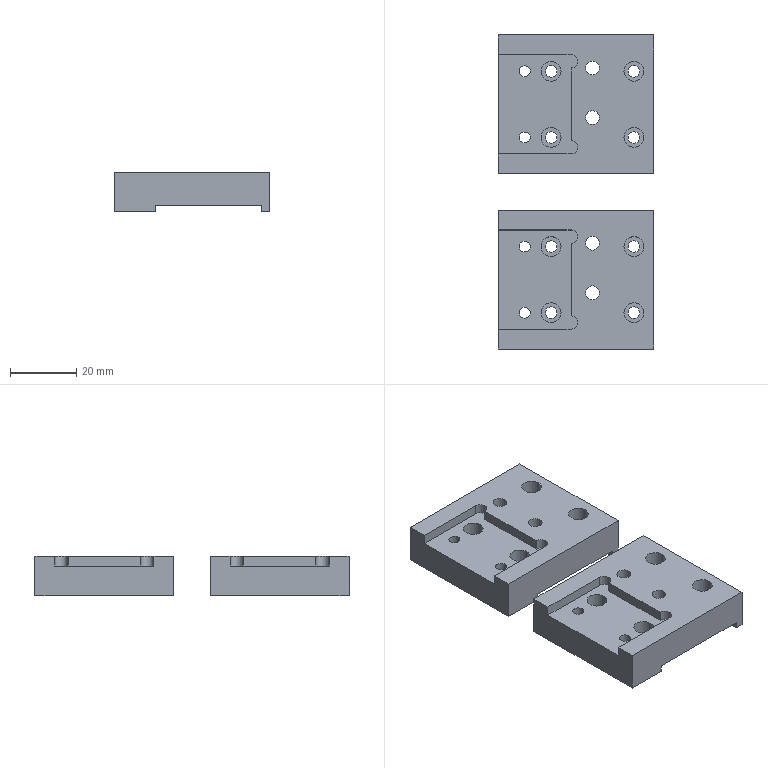NC program | NX | posted with a generic post | part box 47 x 95 x 12 mm
Lines 1783 to 2681 of 2681:
(FLOOR_WALL_COPY , TOOL : D10JING)
N3528 T14 M6
N3530 G54
N3532 G17 G0 G90 X-34.9 Y-30. S9500 M3
N3534 G43 Z30. H14
N3536 Z-1.5
N3538 G94 G1 Z-3. F1500.
N3540 X-35.399 Y-27.634
N3542 G3 X-35.899 Y-28.5 R1.
N3544 G1 Y-7.1
N3546 X-31.199
N3548 Y-28.5
N3550 X-26.5
N3552 Y-7.1
N3554 X-21.8
N3556 Y-28.5
N3558 X-17.1
N3560 Y-7.1
N3562 G3 X-17.966 Y-7.6 R1.
N3564 G1 Z-1.5
N3566 G0 X-18.198 Y-30.
N3568 G1 Z-3.
N3570 X-17.1 Y-29.366
N3572 G3 X-16.6 Y-28.5 R1.
N3574 G1 Y-6.6
N3576 X-36.4
N3578 Y-28.5
N3580 G3 X-35.9 Y-29.366 R1.
N3582 G1 X-34.802 Y-30.
N3584 Z-1.5
N3586 G0 Z0.1
N3588 X18.1
N3590 Z-1.5
N3592 G1 Z-3.
N3594 X17.601 Y-27.634
N3596 G3 X17.101 Y-28.5 R1.
N3598 G1 Y-7.1
N3600 X21.801
N3602 Y-28.5
N3604 X26.5
N3606 Y-7.1
N3608 X31.2
N3610 Y-28.5
N3612 X35.9
N3614 Y-7.1
N3616 G3 X35.034 Y-7.6 R1.
N3618 G1 Z-1.5
N3620 G0 X34.802 Y-30.
N3622 G1 Z-3.
N3624 X35.9 Y-29.366
N3626 G3 X36.4 Y-28.5 R1.
N3628 G1 Y-6.6
N3630 X16.6
N3632 Y-28.5
N3634 G3 X17.1 Y-29.366 R1.
N3636 G1 X18.198 Y-30.
N3638 Z-1.5
N3640 G0 Z30.
(ZLEVEL_PROFILE_COPY_1 , TOOL : D10JING)
N3642 X-0.5 Y-4.296
N3644 Z1.5
N3646 G1 Y-24.049 Z0.465 F1000.
N3648 X-0.828 Y-25.364 Z0.394
N3650 X-1.496 Y-26.545 Z0.323
N3652 X-2.455 Y-27.504 Z0.252
N3654 X-3.636 Y-28.172 Z0.18
N3656 X-4.951 Y-28.5 Z0.109
N3658 X-48.049 Z-2.149
N3660 X-49.364 Y-28.172 Z-2.22
N3662 X-50.545 Y-27.504 Z-2.291
N3664 X-51.504 Y-26.545 Z-2.362
N3666 X-52.172 Y-25.364 Z-2.434
N3668 X-52.5 Y-24.049 Z-2.505
N3670 Y24.049 Z-5.025
N3672 X-52.172 Y25.364 Z-5.096
N3674 X-51.504 Y26.545 Z-5.167
N3676 X-50.545 Y27.504 Z-5.238
N3678 X-49.364 Y28.172 Z-5.31
N3680 X-48.049 Y28.5 Z-5.381
N3682 X-4.951 Z-7.639
N3684 X-3.636 Y28.172 Z-7.71
N3686 X-2.455 Y27.504 Z-7.781
N3688 X-1.496 Y26.545 Z-7.852
N3690 X-0.828 Y25.364 Z-7.924
N3692 X-0.5 Y24.049 Z-7.995
N3694 Y-24.049 Z-10.515
N3696 X-0.828 Y-25.364 Z-10.586
N3698 X-1.496 Y-26.545 Z-10.657
N3700 X-2.455 Y-27.504 Z-10.729
N3702 X-3.636 Y-28.172 Z-10.8
N3704 X-4.951 Y-28.5 Z-10.871
N3706 X-26.5 Z-12.
N3708 X-47.5 F1200.
N3710 G2 X-52.5 Y-23.5 R5.
N3712 G1 Y23.5
N3714 G2 X-47.5 Y28.5 R5.
N3716 G1 X-5.5
N3718 G2 X-0.5 Y23.5 R5.
N3720 G1 Y-23.5
N3722 G2 X-5.5 Y-28.5 R5.
N3724 G1 X-26.5
N3726 Z-10.5
N3728 G0 Z53.
N3730 X52.5 Y-4.296
N3732 Z1.5
N3734 G1 Y-24.049 Z0.465 F1000.
N3736 X52.172 Y-25.364 Z0.394
N3738 X51.504 Y-26.545 Z0.323
N3740 X50.545 Y-27.504 Z0.252
N3742 X49.364 Y-28.172 Z0.18
N3744 X48.049 Y-28.5 Z0.109
N3746 X4.951 Z-2.149
N3748 X3.636 Y-28.172 Z-2.22
N3750 X2.455 Y-27.504 Z-2.291
N3752 X1.496 Y-26.545 Z-2.362
N3754 X0.828 Y-25.364 Z-2.434
N3756 X0.5 Y-24.049 Z-2.505
N3758 Y24.049 Z-5.025
N3760 X0.828 Y25.364 Z-5.096
N3762 X1.496 Y26.545 Z-5.167
N3764 X2.455 Y27.504 Z-5.238
N3766 X3.636 Y28.172 Z-5.31
N3768 X4.951 Y28.5 Z-5.381
N3770 X48.049 Z-7.639
N3772 X49.364 Y28.172 Z-7.71
N3774 X50.545 Y27.504 Z-7.781
N3776 X51.504 Y26.545 Z-7.852
N3778 X52.172 Y25.364 Z-7.924
N3780 X52.5 Y24.049 Z-7.995
N3782 Y-24.049 Z-10.515
N3784 X52.172 Y-25.364 Z-10.586
N3786 X51.504 Y-26.545 Z-10.657
N3788 X50.545 Y-27.504 Z-10.729
N3790 X49.364 Y-28.172 Z-10.8
N3792 X48.049 Y-28.5 Z-10.871
N3794 X26.5 Z-12.
N3796 X5.5 F1200.
N3798 G2 X0.5 Y-23.5 R5.
N3800 G1 Y23.5
N3802 G2 X5.5 Y28.5 R5.
N3804 G1 X47.5
N3806 G2 X52.5 Y23.5 R5.
N3808 G1 Y-23.5
N3810 G2 X47.5 Y-28.5 R5.
N3812 G1 X26.5
N3814 Z-10.5
N3816 G0 Z30.
N3818 M5
(HOLE_MILLING , TOOL : D4)
N3820 T11 M6
N3822 G54
N3824 G17 G0 G90 X-36.5 Y17.5 S9500 M3
N3826 G43 Z30. H11
N3828 Z0.5
N3830 G94 G3 X-36. Y18. R0.5 F1600.
N3832 X-36.5 Y18.5 R0.5
N3834 X-36.5 Y18.5 Z0.1 I0. J-1.
N3836 X-36.5 Y18.5 Z-0.3 I0. J-1.
N3838 X-36.5 Y18.5 Z-0.7 I0. J-1.
N3840 X-36.5 Y18.5 Z-1.1 I0. J-1.
N3842 X-36.5 Y18.5 Z-1.5 I0. J-1.
N3844 X-36.5 Y18.5 Z-1.9 I0. J-1.
N3846 X-36.5 Y18.5 Z-2.3 I0. J-1.
N3848 X-36.5 Y18.5 Z-2.7 I0. J-1.
N3850 X-36.5 Y18.5 Z-3.1 I0. J-1.
N3852 X-36.5 Y18.5 Z-3.5 I0. J-1.
N3854 X-36.5 Y18.5 Z-3.9 I0. J-1.
N3856 X-36.5 Y18.5 Z-4.3 I0. J-1.
N3858 X-36.5 Y18.5 Z-4.7 I0. J-1.
N3860 X-36.5 Y18.5 Z-5.1 I0. J-1.
N3862 X-36.5 Y18.5 Z-5.5 I0. J-1.
N3864 X-36.5 Y18.5 Z-5.9 I0. J-1.
N3866 X-36.5 Y18.5 Z-6.3 I0. J-1.
N3868 X-36.5 Y18.5 Z-6.7 I0. J-1.
N3870 X-36.5 Y18.5 Z-7.1 I0. J-1.
N3872 X-36.5 Y18.5 Z-7.5 I0. J-1.
N3874 X-36.5 Y18.5 Z-7.9 I0. J-1.
N3876 X-37.5 Y17.5 Z-8. R1.
N3878 X-36.5 Y16.5 R1.
N3880 X-37.5 Y17.5 R-1.
N3882 X-37. Y17. R0.5
N3884 X-36.5 Y17.5 R0.5
N3886 G0 Z30.
N3888 Y-7.5
N3890 Z-2.5
N3892 G3 X-36. Y-7. R0.5
N3894 X-36.5 Y-6.5 R0.5
N3896 X-36.5 Y-6.5 Z-2.9 I0. J-1.
N3898 X-36.5 Y-6.5 Z-3.3 I0. J-1.
N3900 X-36.5 Y-6.5 Z-3.7 I0. J-1.
N3902 X-36.5 Y-6.5 Z-4.1 I0. J-1.
N3904 X-36.5 Y-6.5 Z-4.5 I0. J-1.
N3906 X-36.5 Y-6.5 Z-4.9 I0. J-1.
N3908 X-36.5 Y-6.5 Z-5.3 I0. J-1.
N3910 X-36.5 Y-6.5 Z-5.7 I0. J-1.
N3912 X-36.5 Y-6.5 Z-6.1 I0. J-1.
N3914 X-36.5 Y-6.5 Z-6.5 I0. J-1.
N3916 X-36.5 Y-6.5 Z-6.9 I0. J-1.
N3918 X-36.5 Y-6.5 Z-7.3 I0. J-1.
N3920 X-36.5 Y-6.5 Z-7.7 I0. J-1.
N3922 X-35.5 Y-7.5 Z-8. R-1.
N3924 X-36.5 Y-6.5 R1.
N3926 X-35.5 Y-7.5 R-1.
N3928 X-36. Y-7. R0.5
N3930 X-36.5 Y-7.5 R0.5
N3932 G0 Z30.
N3934 X-16.5
N3936 Z-2.5
N3938 G3 X-16. Y-7. R0.5
N3940 X-16.5 Y-6.5 R0.5
N3942 X-16.5 Y-6.5 Z-2.9 I0. J-1.
N3944 X-16.5 Y-6.5 Z-3.3 I0. J-1.
N3946 X-16.5 Y-6.5 Z-3.7 I0. J-1.
N3948 X-16.5 Y-6.5 Z-4.1 I0. J-1.
N3950 X-16.5 Y-6.5 Z-4.5 I0. J-1.
N3952 X-16.5 Y-6.5 Z-4.9 I0. J-1.
N3954 X-16.5 Y-6.5 Z-5.3 I0. J-1.
N3956 X-16.5 Y-6.5 Z-5.7 I0. J-1.
N3958 X-16.5 Y-6.5 Z-6.1 I0. J-1.
N3960 X-16.5 Y-6.5 Z-6.5 I0. J-1.
N3962 X-16.5 Y-6.5 Z-6.9 I0. J-1.
N3964 X-16.5 Y-6.5 Z-7.3 I0. J-1.
N3966 X-16.5 Y-6.5 Z-7.7 I0. J-1.
N3968 X-15.5 Y-7.5 Z-8. R-1.
N3970 X-16.5 Y-6.5 R1.
N3972 X-15.5 Y-7.5 R-1.
N3974 X-16. Y-7. R0.5
N3976 X-16.5 Y-7.5 R0.5
N3978 G0 Z30.
N3980 Y17.5
N3982 Z0.5
N3984 G3 X-16. Y18. R0.5
N3986 X-16.5 Y18.5 R0.5
N3988 X-16.5 Y18.5 Z0.1 I0. J-1.
N3990 X-16.5 Y18.5 Z-0.3 I0. J-1.
N3992 X-16.5 Y18.5 Z-0.7 I0. J-1.
N3994 X-16.5 Y18.5 Z-1.1 I0. J-1.
N3996 X-16.5 Y18.5 Z-1.5 I0. J-1.
N3998 X-16.5 Y18.5 Z-1.9 I0. J-1.
N4000 X-16.5 Y18.5 Z-2.3 I0. J-1.
N4002 X-16.5 Y18.5 Z-2.7 I0. J-1.
N4004 X-16.5 Y18.5 Z-3.1 I0. J-1.
N4006 X-16.5 Y18.5 Z-3.5 I0. J-1.
N4008 X-16.5 Y18.5 Z-3.9 I0. J-1.
N4010 X-16.5 Y18.5 Z-4.3 I0. J-1.
N4012 X-16.5 Y18.5 Z-4.7 I0. J-1.
N4014 X-16.5 Y18.5 Z-5.1 I0. J-1.
N4016 X-16.5 Y18.5 Z-5.5 I0. J-1.
N4018 X-16.5 Y18.5 Z-5.9 I0. J-1.
N4020 X-16.5 Y18.5 Z-6.3 I0. J-1.
N4022 X-16.5 Y18.5 Z-6.7 I0. J-1.
N4024 X-16.5 Y18.5 Z-7.1 I0. J-1.
N4026 X-16.5 Y18.5 Z-7.5 I0. J-1.
N4028 X-16.5 Y18.5 Z-7.9 I0. J-1.
N4030 X-17.5 Y17.5 Z-8. R1.
N4032 X-16.5 Y16.5 R1.
N4034 X-17.5 Y17.5 R-1.
N4036 X-17. Y17. R0.5
N4038 X-16.5 Y17.5 R0.5
N4040 G0 Z30.
N4042 X16.5
N4044 Z0.5
N4046 G3 X17. Y18. R0.5
N4048 X16.5 Y18.5 R0.5
N4050 X16.5 Y18.5 Z0.1 I0. J-1.
N4052 X16.5 Y18.5 Z-0.3 I0. J-1.
N4054 X16.5 Y18.5 Z-0.7 I0. J-1.
N4056 X16.5 Y18.5 Z-1.1 I0. J-1.
N4058 X16.5 Y18.5 Z-1.5 I0. J-1.
N4060 X16.5 Y18.5 Z-1.9 I0. J-1.
N4062 X16.5 Y18.5 Z-2.3 I0. J-1.
N4064 X16.5 Y18.5 Z-2.7 I0. J-1.
N4066 X16.5 Y18.5 Z-3.1 I0. J-1.
N4068 X16.5 Y18.5 Z-3.5 I0. J-1.
N4070 X16.5 Y18.5 Z-3.9 I0. J-1.
N4072 X16.5 Y18.5 Z-4.3 I0. J-1.
N4074 X16.5 Y18.5 Z-4.7 I0. J-1.
N4076 X16.5 Y18.5 Z-5.1 I0. J-1.
N4078 X16.5 Y18.5 Z-5.5 I0. J-1.
N4080 X16.5 Y18.5 Z-5.9 I0. J-1.
N4082 X16.5 Y18.5 Z-6.3 I0. J-1.
N4084 X16.5 Y18.5 Z-6.7 I0. J-1.
N4086 X16.5 Y18.5 Z-7.1 I0. J-1.
N4088 X16.5 Y18.5 Z-7.5 I0. J-1.
N4090 X16.5 Y18.5 Z-7.9 I0. J-1.
N4092 X15.5 Y17.5 Z-8. R1.
N4094 X16.5 Y16.5 R1.
N4096 X15.5 Y17.5 R-1.
N4098 X16. Y17. R0.5
N4100 X16.5 Y17.5 R0.5
N4102 G0 Z30.
N4104 X36.5
N4106 Z0.5
N4108 G3 X37. Y18. R0.5
N4110 X36.5 Y18.5 R0.5
N4112 X36.5 Y18.5 Z0.1 I0. J-1.
N4114 X36.5 Y18.5 Z-0.3 I0. J-1.
N4116 X36.5 Y18.5 Z-0.7 I0. J-1.
N4118 X36.5 Y18.5 Z-1.1 I0. J-1.
N4120 X36.5 Y18.5 Z-1.5 I0. J-1.
N4122 X36.5 Y18.5 Z-1.9 I0. J-1.
N4124 X36.5 Y18.5 Z-2.3 I0. J-1.
N4126 X36.5 Y18.5 Z-2.7 I0. J-1.
N4128 X36.5 Y18.5 Z-3.1 I0. J-1.
N4130 X36.5 Y18.5 Z-3.5 I0. J-1.
N4132 X36.5 Y18.5 Z-3.9 I0. J-1.
N4134 X36.5 Y18.5 Z-4.3 I0. J-1.
N4136 X36.5 Y18.5 Z-4.7 I0. J-1.
N4138 X36.5 Y18.5 Z-5.1 I0. J-1.
N4140 X36.5 Y18.5 Z-5.5 I0. J-1.
N4142 X36.5 Y18.5 Z-5.9 I0. J-1.
N4144 X36.5 Y18.5 Z-6.3 I0. J-1.
N4146 X36.5 Y18.5 Z-6.7 I0. J-1.
N4148 X36.5 Y18.5 Z-7.1 I0. J-1.
N4150 X36.5 Y18.5 Z-7.5 I0. J-1.
N4152 X36.5 Y18.5 Z-7.9 I0. J-1.
N4154 X35.5 Y17.5 Z-8. R1.
N4156 X36.5 Y16.5 R1.
N4158 X35.5 Y17.5 R-1.
N4160 X36. Y17. R0.5
N4162 X36.5 Y17.5 R0.5
N4164 G0 Z30.
N4166 Y-7.5
N4168 Z-2.5
N4170 G3 X37. Y-7. R0.5
N4172 X36.5 Y-6.5 R0.5
N4174 X36.5 Y-6.5 Z-2.9 I0. J-1.
N4176 X36.5 Y-6.5 Z-3.3 I0. J-1.
N4178 X36.5 Y-6.5 Z-3.7 I0. J-1.
N4180 X36.5 Y-6.5 Z-4.1 I0. J-1.
N4182 X36.5 Y-6.5 Z-4.5 I0. J-1.
N4184 X36.5 Y-6.5 Z-4.9 I0. J-1.
N4186 X36.5 Y-6.5 Z-5.3 I0. J-1.
N4188 X36.5 Y-6.5 Z-5.7 I0. J-1.
N4190 X36.5 Y-6.5 Z-6.1 I0. J-1.
N4192 X36.5 Y-6.5 Z-6.5 I0. J-1.
N4194 X36.5 Y-6.5 Z-6.9 I0. J-1.
N4196 X36.5 Y-6.5 Z-7.3 I0. J-1.
N4198 X36.5 Y-6.5 Z-7.7 I0. J-1.
N4200 X37.5 Y-7.5 Z-8. R-1.
N4202 X36.5 Y-6.5 R1.
N4204 X37.5 Y-7.5 R-1.
N4206 X37. Y-7. R0.5
N4208 X36.5 Y-7.5 R0.5
N4210 G0 Z30.
N4212 X16.5
N4214 Z-2.5
N4216 G3 X17. Y-7. R0.5
N4218 X16.5 Y-6.5 R0.5
N4220 X16.5 Y-6.5 Z-2.9 I0. J-1.
N4222 X16.5 Y-6.5 Z-3.3 I0. J-1.
N4224 X16.5 Y-6.5 Z-3.7 I0. J-1.
N4226 X16.5 Y-6.5 Z-4.1 I0. J-1.
N4228 X16.5 Y-6.5 Z-4.5 I0. J-1.
N4230 X16.5 Y-6.5 Z-4.9 I0. J-1.
N4232 X16.5 Y-6.5 Z-5.3 I0. J-1.
N4234 X16.5 Y-6.5 Z-5.7 I0. J-1.
N4236 X16.5 Y-6.5 Z-6.1 I0. J-1.
N4238 X16.5 Y-6.5 Z-6.5 I0. J-1.
N4240 X16.5 Y-6.5 Z-6.9 I0. J-1.
N4242 X16.5 Y-6.5 Z-7.3 I0. J-1.
N4244 X16.5 Y-6.5 Z-7.7 I0. J-1.
N4246 X17.5 Y-7.5 Z-8. R-1.
N4248 X16.5 Y-6.5 R1.
N4250 X17.5 Y-7.5 R-1.
N4252 X17. Y-7. R0.5
N4254 X16.5 Y-7.5 R0.5
N4256 G0 Z30.
(ZLEVEL_PROFILE_COPY , TOOL : D4)
N4258 X38.7 Y-7.09
N4260 Z0.625
N4262 G1 Z-0.375 F1000.
N4264 X39.3 Y-6.743
N4266 G3 X39.5 Y-6.397 R0.4
N4268 G1 Y-1.5 F1500.
N4270 G2 X37.5 Y-3.5 R2.
N4272 G1 X36.603
N4274 G3 X36.257 Y-3.7 R0.4
N4276 G1 X35.91 Y-4.3
N4278 Z0.625
N4280 G0 X38.7 Y-7.09 Z0.25
N4282 G1 Z-0.75 F1000.
N4284 X39.3 Y-6.743
N4286 G3 X39.5 Y-6.397 R0.4
N4288 G1 Y-1.5 F1500.
N4290 G2 X37.5 Y-3.5 R2.
N4292 G1 X36.603
N4294 G3 X36.257 Y-3.7 R0.4
N4296 G1 X35.91 Y-4.3
N4298 Z0.25
N4300 G0 X38.7 Y-7.09 Z-0.125
N4302 G1 Z-1.125 F1000.
N4304 X39.3 Y-6.743
N4306 G3 X39.5 Y-6.397 R0.4
N4308 G1 Y-1.5 F1500.
N4310 G2 X37.5 Y-3.5 R2.
N4312 G1 X36.603
N4314 G3 X36.257 Y-3.7 R0.4
N4316 G1 X35.91 Y-4.3
N4318 Z-0.125
N4320 G0 X38.7 Y-7.09 Z-0.5
N4322 G1 Z-1.5 F1000.
N4324 X39.3 Y-6.743
N4326 G3 X39.5 Y-6.397 R0.4
N4328 G1 Y-1.5 F1500.
N4330 G2 X37.5 Y-3.5 R2.
N4332 G1 X36.603
N4334 G3 X36.257 Y-3.7 R0.4
N4336 G1 X35.91 Y-4.3
N4338 Z-0.5
N4340 G0 X38.7 Y-7.09 Z-0.875
N4342 G1 Z-1.875 F1000.
N4344 X39.3 Y-6.743
N4346 G3 X39.5 Y-6.397 R0.4
N4348 G1 Y-1.5 F1500.
N4350 G2 X37.5 Y-3.5 R2.
N4352 G1 X36.603
N4354 G3 X36.257 Y-3.7 R0.4
N4356 G1 X35.91 Y-4.3
N4358 Z-0.875
N4360 G0 X38.7 Y-7.09 Z-1.25
N4362 G1 Z-2.25 F1000.
N4364 X39.3 Y-6.743
N4366 G3 X39.5 Y-6.397 R0.4
N4368 G1 Y-1.5 F1500.
N4370 G2 X37.5 Y-3.5 R2.
N4372 G1 X36.603
N4374 G3 X36.257 Y-3.7 R0.4
N4376 G1 X35.91 Y-4.3
N4378 Z-1.25
N4380 G0 X38.7 Y-7.09 Z-1.625
N4382 G1 Z-2.625 F1000.
N4384 X39.3 Y-6.743
N4386 G3 X39.5 Y-6.397 R0.4
N4388 G1 Y-1.5 F1500.
N4390 G2 X37.5 Y-3.5 R2.
N4392 G1 X36.603
N4394 G3 X36.257 Y-3.7 R0.4
N4396 G1 X35.91 Y-4.3
N4398 Z-1.625
N4400 G0 X38.7 Y-7.09 Z-2.
N4402 G1 Z-3. F1000.
N4404 X39.3 Y-6.743
N4406 G3 X39.5 Y-6.397 R0.4
N4408 G1 Y-1.5 F1500.
N4410 G2 X37.5 Y-3.5 R2.
N4412 G1 X36.603
N4414 G3 X36.257 Y-3.7 R0.4
N4416 G1 X35.91 Y-4.3
N4418 Z-2.
N4420 G0 Z30.
N4422 X17.09
N4424 Z0.625
N4426 G1 Z-0.375 F1000.
N4428 X16.743 Y-3.7
N4430 G3 X16.397 Y-3.5 R0.4
N4432 G1 X15.5 F1500.
N4434 G2 X13.502 Y-1.579 R2.
N4436 G1 X13.5 Y-2.068
N4438 Y-6.397
N4440 G3 X13.7 Y-6.743 R0.4
N4442 G1 X14.3 Y-7.09
N4444 Z0.625
N4446 G0 X17.09 Y-4.3 Z0.25
N4448 G1 Z-0.75 F1000.
N4450 X16.743 Y-3.7
N4452 G3 X16.397 Y-3.5 R0.4
N4454 G1 X15.5 F1500.
N4456 G2 X13.502 Y-1.579 R2.
N4458 G1 X13.5 Y-2.068
N4460 Y-6.397
N4462 G3 X13.7 Y-6.743 R0.4
N4464 G1 X14.3 Y-7.09
N4466 Z0.25
N4468 G0 X17.09 Y-4.3 Z-0.125
N4470 G1 Z-1.125 F1000.
N4472 X16.743 Y-3.7
N4474 G3 X16.397 Y-3.5 R0.4
N4476 G1 X15.5 F1500.
N4478 G2 X13.502 Y-1.579 R2.
N4480 G1 X13.5 Y-2.068
N4482 Y-6.397
N4484 G3 X13.7 Y-6.743 R0.4
N4486 G1 X14.3 Y-7.09
N4488 Z-0.125
N4490 G0 X17.09 Y-4.3 Z-0.5
N4492 G1 Z-1.5 F1000.
N4494 X16.743 Y-3.7
N4496 G3 X16.397 Y-3.5 R0.4
N4498 G1 X15.5 F1500.
N4500 G2 X13.502 Y-1.579 R2.
N4502 G1 X13.5 Y-2.068
N4504 Y-6.397
N4506 G3 X13.7 Y-6.743 R0.4
N4508 G1 X14.3 Y-7.09
N4510 Z-0.5
N4512 G0 X17.09 Y-4.3 Z-0.875
N4514 G1 Z-1.875 F1000.
N4516 X16.743 Y-3.7
N4518 G3 X16.397 Y-3.5 R0.4
N4520 G1 X15.5 F1500.
N4522 G2 X13.502 Y-1.579 R2.
N4524 G1 X13.5 Y-2.068
N4526 Y-6.397
N4528 G3 X13.7 Y-6.743 R0.4
N4530 G1 X14.3 Y-7.09
N4532 Z-0.875
N4534 G0 X17.09 Y-4.3 Z-1.25
N4536 G1 Z-2.25 F1000.
N4538 X16.743 Y-3.7
N4540 G3 X16.397 Y-3.5 R0.4
N4542 G1 X15.5 F1500.
N4544 G2 X13.502 Y-1.579 R2.
N4546 G1 X13.5 Y-2.068
N4548 Y-6.397
N4550 G3 X13.7 Y-6.743 R0.4
N4552 G1 X14.3 Y-7.09
N4554 Z-1.25
N4556 G0 X17.09 Y-4.3 Z-1.625
N4558 G1 Z-2.625 F1000.
N4560 X16.743 Y-3.7
N4562 G3 X16.397 Y-3.5 R0.4
N4564 G1 X15.5 F1500.
N4566 G2 X13.501 Y-1.549 R2.
N4568 G1 X13.5 Y-2.068
N4570 Y-6.397
N4572 G3 X13.7 Y-6.743 R0.4
N4574 G1 X14.3 Y-7.09
N4576 Z-1.625
N4578 G0 X17.09 Y-4.3 Z-2.
N4580 G1 Z-3. F1000.
N4582 X16.743 Y-3.7
N4584 G3 X16.397 Y-3.5 R0.4
N4586 G1 X15.5 F1500.
N4588 G2 X13.501 Y-1.573 R2.
N4590 G1 X13.5 Y-2.068
N4592 Y-6.397
N4594 G3 X13.7 Y-6.743 R0.4
N4596 G1 X14.3 Y-7.09
N4598 Z-2.
N4600 G0 Z30.
N4602 X-14.3
N4604 Z0.625
N4606 G1 Z-0.375 F1000.
N4608 X-13.7 Y-6.743
N4610 G3 X-13.5 Y-6.397 R0.4
N4612 G1 Y-1.5 F1500.
N4614 G2 X-15.5 Y-3.5 R2.
N4616 G1 X-16.397
N4618 G3 X-16.743 Y-3.7 R0.4
N4620 G1 X-17.09 Y-4.3
N4622 Z0.625
N4624 G0 X-14.3 Y-7.09 Z0.25
N4626 G1 Z-0.75 F1000.
N4628 X-13.7 Y-6.743
N4630 G3 X-13.5 Y-6.397 R0.4
N4632 G1 Y-1.5 F1500.
N4634 G2 X-15.5 Y-3.5 R2.
N4636 G1 X-16.397
N4638 G3 X-16.743 Y-3.7 R0.4
N4640 G1 X-17.09 Y-4.3
N4642 Z0.25
N4644 G0 X-14.3 Y-7.09 Z-0.125
N4646 G1 Z-1.125 F1000.
N4648 X-13.7 Y-6.743
N4650 G3 X-13.5 Y-6.397 R0.4
N4652 G1 Y-1.5 F1500.
N4654 G2 X-15.5 Y-3.5 R2.
N4656 G1 X-16.397
N4658 G3 X-16.743 Y-3.7 R0.4
N4660 G1 X-17.09 Y-4.3
N4662 Z-0.125
N4664 G0 X-14.3 Y-7.09 Z-0.5
N4666 G1 Z-1.5 F1000.
N4668 X-13.7 Y-6.743
N4670 G3 X-13.5 Y-6.397 R0.4
N4672 G1 Y-1.5 F1500.
N4674 G2 X-15.5 Y-3.5 R2.
N4676 G1 X-16.397
N4678 G3 X-16.743 Y-3.7 R0.4
N4680 G1 X-17.09 Y-4.3
N4682 Z-0.5
N4684 G0 X-14.3 Y-7.09 Z-0.875
N4686 G1 Z-1.875 F1000.
N4688 X-13.7 Y-6.743
N4690 G3 X-13.5 Y-6.397 R0.4
N4692 G1 Y-1.5 F1500.
N4694 G2 X-15.5 Y-3.5 R2.
N4696 G1 X-16.397
N4698 G3 X-16.743 Y-3.7 R0.4
N4700 G1 X-17.09 Y-4.3
N4702 Z-0.875
N4704 G0 X-14.3 Y-7.09 Z-1.25
N4706 G1 Z-2.25 F1000.
N4708 X-13.7 Y-6.743
N4710 G3 X-13.5 Y-6.397 R0.4
N4712 G1 Y-1.5 F1500.
N4714 G2 X-15.5 Y-3.5 R2.
N4716 G1 X-16.397
N4718 G3 X-16.743 Y-3.7 R0.4
N4720 G1 X-17.09 Y-4.3
N4722 Z-1.25
N4724 G0 X-14.3 Y-7.09 Z-1.625
N4726 G1 Z-2.625 F1000.
N4728 X-13.7 Y-6.743
N4730 G3 X-13.5 Y-6.397 R0.4
N4732 G1 Y-1.5 F1500.
N4734 G2 X-15.5 Y-3.5 R2.
N4736 G1 X-16.397
N4738 G3 X-16.743 Y-3.7 R0.4
N4740 G1 X-17.09 Y-4.3
N4742 Z-1.625
N4744 G0 X-14.3 Y-7.09 Z-2.
N4746 G1 Z-3. F1000.
N4748 X-13.7 Y-6.743
N4750 G3 X-13.5 Y-6.397 R0.4
N4752 G1 Y-1.5 F1500.
N4754 G2 X-15.5 Y-3.5 R2.
N4756 G1 X-16.397
N4758 G3 X-16.743 Y-3.7 R0.4
N4760 G1 X-17.09 Y-4.3
N4762 Z-2.
N4764 G0 Z30.
N4766 X-35.91
N4768 Z0.625
N4770 G1 Z-0.375 F1000.
N4772 X-36.257 Y-3.7
N4774 G3 X-36.603 Y-3.5 R0.4
N4776 G1 X-37.5 F1500.
N4778 G2 X-39.498 Y-1.579 R2.
N4780 G1 X-39.5 Y-2.068
N4782 Y-6.397
N4784 G3 X-39.3 Y-6.743 R0.4
N4786 G1 X-38.7 Y-7.09
N4788 Z0.625
N4790 G0 X-35.91 Y-4.3 Z0.25
N4792 G1 Z-0.75 F1000.
N4794 X-36.257 Y-3.7
N4796 G3 X-36.603 Y-3.5 R0.4
N4798 G1 X-37.5 F1500.
N4800 G2 X-39.498 Y-1.579 R2.
N4802 G1 X-39.5 Y-2.068
N4804 Y-6.397
N4806 G3 X-39.3 Y-6.743 R0.4
N4808 G1 X-38.7 Y-7.09
N4810 Z0.25
N4812 G0 X-35.91 Y-4.3 Z-0.125
N4814 G1 Z-1.125 F1000.
N4816 X-36.257 Y-3.7
N4818 G3 X-36.603 Y-3.5 R0.4
N4820 G1 X-37.5 F1500.
N4822 G2 X-39.498 Y-1.579 R2.
N4824 G1 X-39.5 Y-2.068
N4826 Y-6.397
N4828 G3 X-39.3 Y-6.743 R0.4
N4830 G1 X-38.7 Y-7.09
N4832 Z-0.125
N4834 G0 X-35.91 Y-4.3 Z-0.5
N4836 G1 Z-1.5 F1000.
N4838 X-36.257 Y-3.7
N4840 G3 X-36.603 Y-3.5 R0.4
N4842 G1 X-37.5 F1500.
N4844 G2 X-39.498 Y-1.579 R2.
N4846 G1 X-39.5 Y-2.068
N4848 Y-6.397
N4850 G3 X-39.3 Y-6.743 R0.4
N4852 G1 X-38.7 Y-7.09
N4854 Z-0.5
N4856 G0 X-35.91 Y-4.3 Z-0.875
N4858 G1 Z-1.875 F1000.
N4860 X-36.257 Y-3.7
N4862 G3 X-36.603 Y-3.5 R0.4
N4864 G1 X-37.5 F1500.
N4866 G2 X-39.498 Y-1.579 R2.
N4868 G1 X-39.5 Y-2.068
N4870 Y-6.397
N4872 G3 X-39.3 Y-6.743 R0.4
N4874 G1 X-38.7 Y-7.09
N4876 Z-0.875
N4878 G0 X-35.91 Y-4.3 Z-1.25
N4880 G1 Z-2.25 F1000.
N4882 X-36.257 Y-3.7
N4884 G3 X-36.603 Y-3.5 R0.4
N4886 G1 X-37.5 F1500.
N4888 G2 X-39.498 Y-1.579 R2.
N4890 G1 X-39.5 Y-2.068
N4892 Y-6.397
N4894 G3 X-39.3 Y-6.743 R0.4
N4896 G1 X-38.7 Y-7.09
N4898 Z-1.25
N4900 G0 X-35.91 Y-4.3 Z-1.625
N4902 G1 Z-2.625 F1000.
N4904 X-36.257 Y-3.7
N4906 G3 X-36.603 Y-3.5 R0.4
N4908 G1 X-37.5 F1500.
N4910 G2 X-39.499 Y-1.549 R2.
N4912 G1 X-39.5 Y-2.068
N4914 Y-6.397
N4916 G3 X-39.3 Y-6.743 R0.4
N4918 G1 X-38.7 Y-7.09
N4920 Z-1.625
N4922 G0 X-35.91 Y-4.3 Z-2.
N4924 G1 Z-3. F1000.
N4926 X-36.257 Y-3.7
N4928 G3 X-36.603 Y-3.5 R0.4
N4930 G1 X-37.5 F1500.
N4932 G2 X-39.499 Y-1.573 R2.
N4934 G1 X-39.5 Y-2.068
N4936 Y-6.397
N4938 G3 X-39.3 Y-6.743 R0.4
N4940 G1 X-38.7 Y-7.09
N4942 Z-2.
N4944 G0 Z30.
N4946 M5
(PLANAR_MILL_COPY_COPY_COPY , TOOL : D6A45)
N4948 T01 M6
N4950 G54
N4952 G17 G0 G90 X-35.634 Y19.1 S9500 M3
N4954 G43 Z30. H1
N4956 Z0.5
N4958 G94 G1 Z-1. F1250.
N4960 G3 X-36.5 Y19.6 R1.
N4962 X-38.6 Y17.5 R2.1
N4964 X-36.5 Y19.6 R-2.1
N4966 X-37.366 Y19.1 R1.
N4968 G1 Z0.5
N4970 G0 Z30.
N4972 X-38.2 Y5.866
N4974 Z0.5
N4976 G1 Z-1.
N4978 G3 X-38.7 Y5. R1.
N4980 X-37.5 Y3.8 R1.2
N4982 X-38.7 Y5. R-1.2
N4984 X-38.2 Y4.134 R1.
N4986 G1 Z0.5
N4988 G0 Z30.
N4990 X-48.9 Y-0.866
N4992 Z0.5
N4994 G1 Z-1.
N4996 G3 X-48.4 Y0. R1.
N4998 G1 Y23.5
N5000 G2 X-47.5 Y24.4 R0.9
N5002 G1 X-5.5
N5004 G2 X-4.6 Y23.5 R0.9
N5006 G1 Y-23.5
N5008 G2 X-5.5 Y-24.4 R0.9
N5010 G1 X-11.5
N5012 G2 X-12.4 Y-23.5 R0.9
N5014 G1 Y-1.5
N5016 G3 X-13.5 Y-0.4 R1.1
N5018 X-14.6 Y-1.5 R1.1
N5020 G2 X-15.5 Y-2.4 R0.9
N5022 G1 X-37.5
N5024 G2 X-38.4 Y-1.5 R0.9
N5026 G3 X-39.5 Y-0.4 R1.1
N5028 X-40.6 Y-1.5 R1.1
N5030 G1 Y-23.5
N5032 G2 X-41.5 Y-24.4 R0.9
N5034 G1 X-47.5
N5036 G2 X-48.4 Y-23.5 R0.9
N5038 G1 Y0.
N5040 G3 X-48.9 Y0.866 R1.
N5042 G1 Z0.5
N5044 G0 Z30.
N5046 X-21.634 Y5.7
N5048 Z0.5
N5050 G1 Z-1.
N5052 G3 X-22.5 Y6.2 R1.
N5054 X-23.7 Y5. R1.2
N5056 X-22.5 Y6.2 R-1.2
N5058 X-23.366 Y5.7 R1.
N5060 G1 Z0.5
N5062 G0 Z30.
N5064 X-15.634 Y19.1
N5066 Z0.5
N5068 G1 Z-1.
N5070 G3 X-16.5 Y19.6 R1.
N5072 X-18.6 Y17.5 R2.1
N5074 X-16.5 Y19.6 R-2.1
N5076 X-17.366 Y19.1 R1.
N5078 G1 Z0.5
N5080 G0 Z30.
N5082 X17.366
N5084 Z0.5
N5086 G1 Z-1.
N5088 G3 X16.5 Y19.6 R1.
N5090 X14.4 Y17.5 R2.1
N5092 X16.5 Y19.6 R-2.1
N5094 X15.634 Y19.1 R1.
N5096 G1 Z0.5
N5098 G0 Z30.
N5100 X16.366 Y5.7
N5102 Z0.5
N5104 G1 Z-1.
N5106 G3 X15.5 Y6.2 R1.
N5108 X14.3 Y5. R1.2
N5110 X15.5 Y6.2 R-1.2
N5112 X14.634 Y5.7 R1.
N5114 G1 Z0.5
N5116 G0 Z30.
N5118 X48.9 Y0.866
N5120 Z0.5
N5122 G1 Z-1.
N5124 G3 X48.4 Y0. R1.
N5126 G1 Y-23.5
N5128 G2 X47.5 Y-24.4 R0.9
N5130 G1 X41.5
N5132 G2 X40.6 Y-23.5 R0.9
N5134 G1 Y-1.5
N5136 G3 X39.5 Y-0.4 R1.1
N5138 X38.4 Y-1.5 R1.1
N5140 G2 X37.5 Y-2.4 R0.9
N5142 G1 X15.5
N5144 G2 X14.6 Y-1.5 R0.9
N5146 G3 X13.5 Y-0.4 R1.1
N5148 X12.4 Y-1.5 R1.1
N5150 G1 Y-23.5
N5152 G2 X11.5 Y-24.4 R0.9
N5154 G1 X5.5
N5156 G2 X4.6 Y-23.5 R0.9
N5158 G1 Y23.5
N5160 G2 X5.5 Y24.4 R0.9
N5162 G1 X47.5
N5164 G2 X48.4 Y23.5 R0.9
N5166 G1 Y0.
N5168 G3 X48.9 Y-0.866 R1.
N5170 G1 Z0.5
N5172 G0 Z30.
N5174 X31.2 Y4.134
N5176 Z0.5
N5178 G1 Z-1.
N5180 G3 X31.7 Y5. R1.
N5182 X30.5 Y6.2 R1.2
N5184 X31.7 Y5. R-1.2
N5186 X31.2 Y5.866 R1.
N5188 G1 Z0.5
N5190 G0 Z30.
N5192 X37.366 Y19.1
N5194 Z0.5
N5196 G1 Z-1.
N5198 G3 X36.5 Y19.6 R1.
N5200 X34.4 Y17.5 R2.1
N5202 X36.5 Y19.6 R-2.1
N5204 X35.634 Y19.1 R1.
N5206 G1 Z0.5
N5208 G0 Z30.
N5210 M5
(刀补 , TOOL : D4)
N5212 T11 M6
N5214 G54
N5216 G17 G0 G90 X-15.144 Y-26.631 S9500 M3
N5218 G43 Z30. H11
N5220 Z-1.5
N5222 G94 G1 Z-3. F1500.
N5224 G41 X-15.05 Y-26.597 D11
N5226 X-13.75 Y-25.846
N5228 G3 X-13.55 Y-25.5 R0.4
N5230 G1 Y-2.132
N5232 G2 X-15.5 Y-3.55 R2.05
N5234 G1 X-37.5
N5236 G2 X-39.45 Y-2.132 R2.05
N5238 G1 Y-25.5
N5240 G3 X-39.25 Y-25.846 R0.4
N5242 G1 X-37.95 Y-26.597
N5244 G40
N5246 X-37.856 Y-26.631
N5248 Z-1.5
N5250 G0 Z0.1
N5252 X37.856
N5254 Z-1.5
N5256 G1 Z-3.
N5258 G41 X37.95 Y-26.597
N5260 X39.25 Y-25.846
N5262 G3 X39.45 Y-25.5 R0.4
N5264 G1 Y-2.132
N5266 G2 X37.5 Y-3.55 R2.05
N5268 G1 X15.5
N5270 G2 X13.55 Y-2.132 R2.05
N5272 G1 Y-25.5
N5274 G3 X13.75 Y-25.846 R0.4
N5276 G1 X15.05 Y-26.597
N5278 G40
N5280 X15.144 Y-26.631
N5282 Z-1.5
N5284 G0 Z30.
N5286 M5
N5288 M2